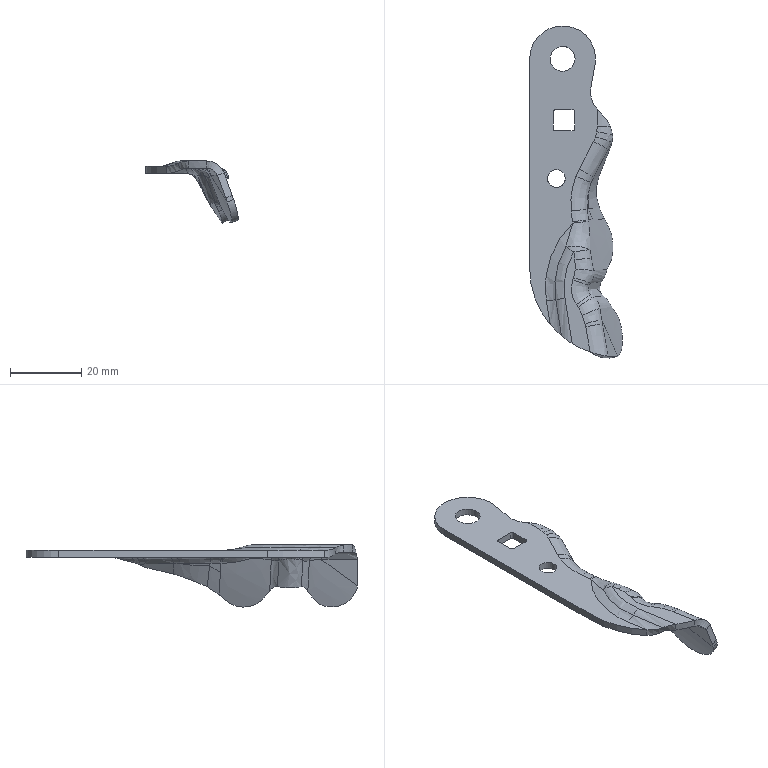Part | STEP file | 1 solid | 120 faces | box 26.045 x 93.231 x 17.45 mm | volume 4101 mm3 | spline 96 | cylinder 11 | plane 10 | sphere 2 | other 1 | commonest cylinder face diameters 1 x4 5 x1 6 x1 7 x1 10 x1 13.815 x1